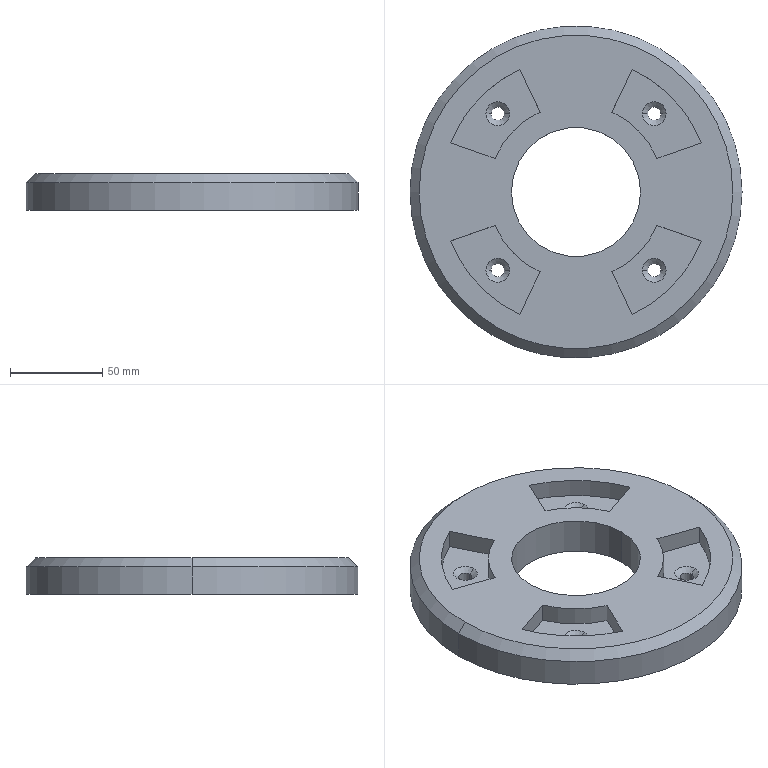Part | SolidWorks | features MirrorPattern 2, Chamfer 1, Extrusion 1, HoleWzd 1, ICE 1 | 1 solid | 44 faces | box 180 x 180 x 20 mm | volume 376159 mm3 | cylinder 20 | plane 14 | cone 10 | commonest cylinder face diameters 7.142 x8 95 x4 146.043 x4 70 x2 180 x2
STEP:
#1=CARTESIAN_POINT('',(38.855,-42.426,7.594));
#2=VERTEX_POINT('',#1);
#3=CARTESIAN_POINT('',(45.998,-42.426,7.594));
#4=VERTEX_POINT('',#3);
#5=CARTESIAN_POINT('',(42.426,-42.426,7.594));
#6=DIRECTION('',(0.,0.,1.));
#7=DIRECTION('',(1.,0.,0.));
#8=AXIS2_PLACEMENT_3D('',#5,#6,#7);
#9=CIRCLE('',#8,3.571);
#10=EDGE_CURVE('',#2,#4,#9,.T.);
#11=ORIENTED_EDGE('',*,*,#10,.F.);
#12=CARTESIAN_POINT('',(35.988,-42.426,10.));
#13=VERTEX_POINT('',#12);
#14=CARTESIAN_POINT('',(35.988,-42.426,10.));
#15=DIRECTION('',(-0.766,0.,0.6428));
#16=VECTOR('',#15,1000.);
#17=LINE('',#14,#16);
#18=EDGE_CURVE('',#2,#13,#17,.T.);
#19=ORIENTED_EDGE('',*,*,#18,.T.);
#20=CARTESIAN_POINT('',(48.865,-42.426,10.));
#21=VERTEX_POINT('',#20);
#22=CARTESIAN_POINT('',(42.426,-42.426,10.));
#23=DIRECTION('',(0.,0.,1.));
#24=DIRECTION('',(1.,0.,0.));
#25=AXIS2_PLACEMENT_3D('',#22,#23,#24);
#26=CIRCLE('',#25,6.439);
#27=EDGE_CURVE('',#13,#21,#26,.T.);
#28=ORIENTED_EDGE('',*,*,#27,.T.);
#29=CARTESIAN_POINT('',(48.865,-42.426,10.));
#30=DIRECTION('',(0.766,0.,0.6428));
#31=VECTOR('',#30,1000.);
#32=LINE('',#29,#31);
#33=EDGE_CURVE('',#4,#21,#32,.T.);
#34=ORIENTED_EDGE('',*,*,#33,.F.);
#35=EDGE_LOOP('',(#11,#19,#28,#34));
#36=FACE_OUTER_BOUND('',#35,.T.);
#37=CARTESIAN_POINT('',(42.426,-42.426,10.));
#38=DIRECTION('',(0.,0.,1.));
#39=DIRECTION('',(1.,0.,0.));
#40=AXIS2_PLACEMENT_3D('',#37,#38,#39);
#41=CONICAL_SURFACE('',#40,6.439,0.8727);
#42=ADVANCED_FACE('',(#36),#41,.F.);
#43=CARTESIAN_POINT('',(38.855,-42.426,0.));
#44=VERTEX_POINT('',#43);
#45=CARTESIAN_POINT('',(45.998,-42.426,0.));
#46=VERTEX_POINT('',#45);
#47=CARTESIAN_POINT('',(42.426,-42.426,0.));
#48=DIRECTION('',(0.,0.,1.));
#49=DIRECTION('',(1.,0.,0.));
#50=AXIS2_PLACEMENT_3D('',#47,#48,#49);
#51=CIRCLE('',#50,3.571);
#52=EDGE_CURVE('',#44,#46,#51,.T.);
#53=ORIENTED_EDGE('',*,*,#52,.F.);
#54=CARTESIAN_POINT('',(38.855,-42.426,10.));
#55=DIRECTION('',(0.,0.,1.));
#56=VECTOR('',#55,1000.);
#57=LINE('',#54,#56);
#58=EDGE_CURVE('',#44,#2,#57,.T.);
#59=ORIENTED_EDGE('',*,*,#58,.T.);
#60=ORIENTED_EDGE('',*,*,#10,.T.);
#61=CARTESIAN_POINT('',(45.998,-42.426,10.));
#62=DIRECTION('',(0.,0.,1.));
#63=VECTOR('',#62,1000.);
#64=LINE('',#61,#63);
#65=EDGE_CURVE('',#46,#4,#64,.T.);
#66=ORIENTED_EDGE('',*,*,#65,.F.);
#67=EDGE_LOOP('',(#53,#59,#60,#66));
#68=FACE_OUTER_BOUND('',#67,.T.);
#69=CARTESIAN_POINT('',(42.426,-42.426,10.));
#70=DIRECTION('',(0.,0.,1.));
#71=DIRECTION('',(1.,0.,0.));
#72=AXIS2_PLACEMENT_3D('',#69,#70,#71);
#73=CYLINDRICAL_SURFACE('',#72,3.571);
#74=ADVANCED_FACE('',(#68),#73,.F.);
#75=CARTESIAN_POINT('',(-45.998,-42.426,7.594));
#76=VERTEX_POINT('',#75);
#77=CARTESIAN_POINT('',(-38.855,-42.426,7.594));
#78=VERTEX_POINT('',#77);
#79=CARTESIAN_POINT('',(-42.426,-42.426,7.594));
#80=DIRECTION('',(0.,0.,1.));
#81=DIRECTION('',(1.,0.,0.));
#82=AXIS2_PLACEMENT_3D('',#79,#80,#81);
#83=CIRCLE('',#82,3.571);
#84=EDGE_CURVE('',#76,#78,#83,.T.);
#85=ORIENTED_EDGE('',*,*,#84,.F.);
#86=CARTESIAN_POINT('',(-48.865,-42.426,10.));
#87=VERTEX_POINT('',#86);
#88=CARTESIAN_POINT('',(-48.865,-42.426,10.));
#89=DIRECTION('',(-0.766,0.,0.6428));
#90=VECTOR('',#89,1000.);
#91=LINE('',#88,#90);
#92=EDGE_CURVE('',#76,#87,#91,.T.);
#93=ORIENTED_EDGE('',*,*,#92,.T.);
#94=CARTESIAN_POINT('',(-35.988,-42.426,10.));
#95=VERTEX_POINT('',#94);
#96=CARTESIAN_POINT('',(-42.426,-42.426,10.));
#97=DIRECTION('',(0.,0.,1.));
#98=DIRECTION('',(1.,0.,0.));
#99=AXIS2_PLACEMENT_3D('',#96,#97,#98);
#100=CIRCLE('',#99,6.439);
#101=EDGE_CURVE('',#87,#95,#100,.T.);
#102=ORIENTED_EDGE('',*,*,#101,.T.);
#103=CARTESIAN_POINT('',(-35.988,-42.426,10.));
#104=DIRECTION('',(0.766,0.,0.6428));
#105=VECTOR('',#104,1000.);
#106=LINE('',#103,#105);
#107=EDGE_CURVE('',#78,#95,#106,.T.);
#108=ORIENTED_EDGE('',*,*,#107,.F.);
#109=EDGE_LOOP('',(#85,#93,#102,#108));
#110=FACE_OUTER_BOUND('',#109,.T.);
#111=CARTESIAN_POINT('',(-42.426,-42.426,10.));
#112=DIRECTION('',(0.,0.,1.));
#113=DIRECTION('',(1.,0.,0.));
#114=AXIS2_PLACEMENT_3D('',#111,#112,#113);
#115=CONICAL_SURFACE('',#114,6.439,0.8727);
#116=ADVANCED_FACE('',(#110),#115,.F.);
#117=CARTESIAN_POINT('',(-45.998,-42.426,0.));
#118=VERTEX_POINT('',#117);
#119=CARTESIAN_POINT('',(-38.855,-42.426,0.));
#120=VERTEX_POINT('',#119);
#121=CARTESIAN_POINT('',(-42.426,-42.426,0.));
#122=DIRECTION('',(0.,0.,1.));
#123=DIRECTION('',(1.,0.,0.));
#124=AXIS2_PLACEMENT_3D('',#121,#122,#123);
#125=CIRCLE('',#124,3.571);
#126=EDGE_CURVE('',#118,#120,#125,.T.);
#127=ORIENTED_EDGE('',*,*,#126,.F.);
#128=CARTESIAN_POINT('',(-45.998,-42.426,10.));
#129=DIRECTION('',(0.,0.,1.));
#130=VECTOR('',#129,1000.);
#131=LINE('',#128,#130);
#132=EDGE_CURVE('',#118,#76,#131,.T.);
#133=ORIENTED_EDGE('',*,*,#132,.T.);
#134=ORIENTED_EDGE('',*,*,#84,.T.);
#135=CARTESIAN_POINT('',(-38.855,-42.426,10.));
#136=DIRECTION('',(0.,0.,1.));
#137=VECTOR('',#136,1000.);
#138=LINE('',#135,#137);
#139=EDGE_CURVE('',#120,#78,#138,.T.);
#140=ORIENTED_EDGE('',*,*,#139,.F.);
#141=EDGE_LOOP('',(#127,#133,#134,#140));
#142=FACE_OUTER_BOUND('',#141,.T.);
#143=CARTESIAN_POINT('',(-42.426,-42.426,10.));
#144=DIRECTION('',(0.,0.,1.));
#145=DIRECTION('',(1.,0.,0.));
#146=AXIS2_PLACEMENT_3D('',#143,#144,#145);
#147=CYLINDRICAL_SURFACE('',#146,3.571);
#148=ADVANCED_FACE('',(#142),#147,.F.);
#149=CARTESIAN_POINT('',(38.855,42.426,7.594));
#150=VERTEX_POINT('',#149);
#151=CARTESIAN_POINT('',(45.998,42.426,7.594));
#152=VERTEX_POINT('',#151);
#153=CARTESIAN_POINT('',(42.426,42.426,7.594));
#154=DIRECTION('',(0.,0.,1.));
#155=DIRECTION('',(1.,0.,0.));
#156=AXIS2_PLACEMENT_3D('',#153,#154,#155);
#157=CIRCLE('',#156,3.571);
#158=EDGE_CURVE('',#150,#152,#157,.T.);
#159=ORIENTED_EDGE('',*,*,#158,.F.);
#160=CARTESIAN_POINT('',(35.988,42.426,10.));
#161=VERTEX_POINT('',#160);
#162=CARTESIAN_POINT('',(35.988,42.426,10.));
#163=DIRECTION('',(-0.766,0.,0.6428));
#164=VECTOR('',#163,1000.);
#165=LINE('',#162,#164);
#166=EDGE_CURVE('',#150,#161,#165,.T.);
#167=ORIENTED_EDGE('',*,*,#166,.T.);
#168=CARTESIAN_POINT('',(48.865,42.426,10.));
#169=VERTEX_POINT('',#168);
#170=CARTESIAN_POINT('',(42.426,42.426,10.));
#171=DIRECTION('',(0.,0.,1.));
#172=DIRECTION('',(1.,0.,0.));
#173=AXIS2_PLACEMENT_3D('',#170,#171,#172);
#174=CIRCLE('',#173,6.439);
#175=EDGE_CURVE('',#161,#169,#174,.T.);
#176=ORIENTED_EDGE('',*,*,#175,.T.);
#177=CARTESIAN_POINT('',(48.865,42.426,10.));
#178=DIRECTION('',(0.766,0.,0.6428));
#179=VECTOR('',#178,1000.);
#180=LINE('',#177,#179);
#181=EDGE_CURVE('',#152,#169,#180,.T.);
#182=ORIENTED_EDGE('',*,*,#181,.F.);
#183=EDGE_LOOP('',(#159,#167,#176,#182));
#184=FACE_OUTER_BOUND('',#183,.T.);
#185=CARTESIAN_POINT('',(42.426,42.426,10.));
#186=DIRECTION('',(0.,0.,1.));
#187=DIRECTION('',(1.,0.,0.));
#188=AXIS2_PLACEMENT_3D('',#185,#186,#187);
#189=CONICAL_SURFACE('',#188,6.439,0.8727);
#190=ADVANCED_FACE('',(#184),#189,.F.);
#191=CARTESIAN_POINT('',(38.855,42.426,0.));
#192=VERTEX_POINT('',#191);
#193=CARTESIAN_POINT('',(45.998,42.426,0.));
#194=VERTEX_POINT('',#193);
#195=CARTESIAN_POINT('',(42.426,42.426,0.));
#196=DIRECTION('',(0.,0.,1.));
#197=DIRECTION('',(1.,0.,0.));
#198=AXIS2_PLACEMENT_3D('',#195,#196,#197);
#199=CIRCLE('',#198,3.571);
#200=EDGE_CURVE('',#192,#194,#199,.T.);
#201=ORIENTED_EDGE('',*,*,#200,.F.);
#202=CARTESIAN_POINT('',(38.855,42.426,10.));
#203=DIRECTION('',(0.,0.,1.));
#204=VECTOR('',#203,1000.);
#205=LINE('',#202,#204);
#206=EDGE_CURVE('',#192,#150,#205,.T.);
#207=ORIENTED_EDGE('',*,*,#206,.T.);
#208=ORIENTED_EDGE('',*,*,#158,.T.);
#209=CARTESIAN_POINT('',(45.998,42.426,10.));
#210=DIRECTION('',(0.,0.,1.));
#211=VECTOR('',#210,1000.);
#212=LINE('',#209,#211);
#213=EDGE_CURVE('',#194,#152,#212,.T.);
#214=ORIENTED_EDGE('',*,*,#213,.F.);
#215=EDGE_LOOP('',(#201,#207,#208,#214));
#216=FACE_OUTER_BOUND('',#215,.T.);
#217=CARTESIAN_POINT('',(42.426,42.426,10.));
#218=DIRECTION('',(0.,0.,1.));
#219=DIRECTION('',(1.,0.,0.));
#220=AXIS2_PLACEMENT_3D('',#217,#218,#219);
#221=CYLINDRICAL_SURFACE('',#220,3.571);
#222=ADVANCED_FACE('',(#216),#221,.F.);
#223=CARTESIAN_POINT('',(-45.998,42.426,7.594));
#224=VERTEX_POINT('',#223);
#225=CARTESIAN_POINT('',(-38.855,42.426,7.594));
#226=VERTEX_POINT('',#225);
#227=CARTESIAN_POINT('',(-42.426,42.426,7.594));
#228=DIRECTION('',(0.,0.,1.));
#229=DIRECTION('',(1.,0.,0.));
#230=AXIS2_PLACEMENT_3D('',#227,#228,#229);
#231=CIRCLE('',#230,3.571);
#232=EDGE_CURVE('',#224,#226,#231,.T.);
#233=ORIENTED_EDGE('',*,*,#232,.F.);
#234=CARTESIAN_POINT('',(-48.865,42.426,10.));
#235=VERTEX_POINT('',#234);
#236=CARTESIAN_POINT('',(-48.865,42.426,10.));
#237=DIRECTION('',(-0.766,0.,0.6428));
#238=VECTOR('',#237,1000.);
#239=LINE('',#236,#238);
#240=EDGE_CURVE('',#224,#235,#239,.T.);
#241=ORIENTED_EDGE('',*,*,#240,.T.);
#242=CARTESIAN_POINT('',(-35.988,42.426,10.));
#243=VERTEX_POINT('',#242);
#244=CARTESIAN_POINT('',(-42.426,42.426,10.));
#245=DIRECTION('',(0.,0.,1.));
#246=DIRECTION('',(1.,0.,0.));
#247=AXIS2_PLACEMENT_3D('',#244,#245,#246);
#248=CIRCLE('',#247,6.439);
#249=EDGE_CURVE('',#235,#243,#248,.T.);
#250=ORIENTED_EDGE('',*,*,#249,.T.);
#251=CARTESIAN_POINT('',(-35.988,42.426,10.));
#252=DIRECTION('',(0.766,0.,0.6428));
#253=VECTOR('',#252,1000.);
#254=LINE('',#251,#253);
#255=EDGE_CURVE('',#226,#243,#254,.T.);
#256=ORIENTED_EDGE('',*,*,#255,.F.);
#257=EDGE_LOOP('',(#233,#241,#250,#256));
#258=FACE_OUTER_BOUND('',#257,.T.);
#259=CARTESIAN_POINT('',(-42.426,42.426,10.));
#260=DIRECTION('',(0.,0.,1.));
#261=DIRECTION('',(1.,0.,0.));
#262=AXIS2_PLACEMENT_3D('',#259,#260,#261);
#263=CONICAL_SURFACE('',#262,6.439,0.8727);
#264=ADVANCED_FACE('',(#258),#263,.F.);
#265=CARTESIAN_POINT('',(-45.998,42.426,0.));
#266=VERTEX_POINT('',#265);
#267=CARTESIAN_POINT('',(-38.855,42.426,0.));
#268=VERTEX_POINT('',#267);
#269=CARTESIAN_POINT('',(-42.426,42.426,0.));
#270=DIRECTION('',(0.,0.,1.));
#271=DIRECTION('',(1.,0.,0.));
#272=AXIS2_PLACEMENT_3D('',#269,#270,#271);
#273=CIRCLE('',#272,3.571);
#274=EDGE_CURVE('',#266,#268,#273,.T.);
#275=ORIENTED_EDGE('',*,*,#274,.F.);
#276=CARTESIAN_POINT('',(-45.998,42.426,10.));
#277=DIRECTION('',(0.,0.,1.));
#278=VECTOR('',#277,1000.);
#279=LINE('',#276,#278);
#280=EDGE_CURVE('',#266,#224,#279,.T.);
#281=ORIENTED_EDGE('',*,*,#280,.T.);
#282=ORIENTED_EDGE('',*,*,#232,.T.);
#283=CARTESIAN_POINT('',(-38.855,42.426,10.));
#284=DIRECTION('',(0.,0.,1.));
#285=VECTOR('',#284,1000.);
#286=LINE('',#283,#285);
#287=EDGE_CURVE('',#268,#226,#286,.T.);
#288=ORIENTED_EDGE('',*,*,#287,.F.);
#289=EDGE_LOOP('',(#275,#281,#282,#288));
#290=FACE_OUTER_BOUND('',#289,.T.);
#291=CARTESIAN_POINT('',(-42.426,42.426,10.));
#292=DIRECTION('',(0.,0.,1.));
#293=DIRECTION('',(1.,0.,0.));
#294=AXIS2_PLACEMENT_3D('',#291,#292,#293);
#295=CYLINDRICAL_SURFACE('',#294,3.571);
#296=ADVANCED_FACE('',(#290),#295,.F.);
#297=CARTESIAN_POINT('',(85.,0.,20.));
#298=VERTEX_POINT('',#297);
#299=CARTESIAN_POINT('',(-85.,0.,20.));
#300=VERTEX_POINT('',#299);
#301=CARTESIAN_POINT('',(0.,0.,20.));
#302=DIRECTION('',(0.,0.,1.));
#303=DIRECTION('',(1.,0.,0.));
#304=AXIS2_PLACEMENT_3D('',#301,#302,#303);
#305=CIRCLE('',#304,85.);
#306=EDGE_CURVE('',#298,#300,#305,.T.);
#307=ORIENTED_EDGE('',*,*,#306,.F.);
#308=CARTESIAN_POINT('',(90.,0.,15.));
#309=VERTEX_POINT('',#308);
#310=CARTESIAN_POINT('',(85.,0.,20.));
#311=DIRECTION('',(0.7071,0.,-0.7071));
#312=VECTOR('',#311,1000.);
#313=LINE('',#310,#312);
#314=EDGE_CURVE('',#298,#309,#313,.T.);
#315=ORIENTED_EDGE('',*,*,#314,.T.);
#316=CARTESIAN_POINT('',(-90.,0.,15.));
#317=VERTEX_POINT('',#316);
#318=CARTESIAN_POINT('',(0.,0.,15.));
#319=DIRECTION('',(0.,0.,-1.));
#320=DIRECTION('',(1.,0.,0.));
#321=AXIS2_PLACEMENT_3D('',#318,#319,#320);
#322=CIRCLE('',#321,90.);
#323=EDGE_CURVE('',#317,#309,#322,.T.);
#324=ORIENTED_EDGE('',*,*,#323,.F.);
#325=CARTESIAN_POINT('',(-85.,0.,20.));
#326=DIRECTION('',(-0.7071,0.,-0.7071));
#327=VECTOR('',#326,1000.);
#328=LINE('',#325,#327);
#329=EDGE_CURVE('',#300,#317,#328,.T.);
#330=ORIENTED_EDGE('',*,*,#329,.F.);
#331=EDGE_LOOP('',(#307,#315,#324,#330));
#332=FACE_OUTER_BOUND('',#331,.T.);
#333=CARTESIAN_POINT('',(0.,0.,20.));
#334=DIRECTION('',(0.,0.,-1.));
#335=DIRECTION('',(-1.,0.,0.));
#336=AXIS2_PLACEMENT_3D('',#333,#334,#335);
#337=CONICAL_SURFACE('',#336,85.,0.7854);
#338=ADVANCED_FACE('',(#332),#337,.T.);
#339=CARTESIAN_POINT('',(-35.,0.,20.));
#340=VERTEX_POINT('',#339);
#341=CARTESIAN_POINT('',(35.,0.,20.));
#342=VERTEX_POINT('',#341);
#343=CARTESIAN_POINT('',(0.,0.,20.));
#344=DIRECTION('',(0.,0.,1.));
#345=DIRECTION('',(1.,0.,0.));
#346=AXIS2_PLACEMENT_3D('',#343,#344,#345);
#347=CIRCLE('',#346,35.);
#348=EDGE_CURVE('',#340,#342,#347,.T.);
#349=ORIENTED_EDGE('',*,*,#348,.T.);
#350=CARTESIAN_POINT('',(35.,0.,0.));
#351=VERTEX_POINT('',#350);
#352=CARTESIAN_POINT('',(35.,0.,20.));
#353=DIRECTION('',(0.,0.,-1.));
#354=VECTOR('',#353,1000.);
#355=LINE('',#352,#354);
#356=EDGE_CURVE('',#342,#351,#355,.T.);
#357=ORIENTED_EDGE('',*,*,#356,.T.);
#358=CARTESIAN_POINT('',(-35.,0.,0.));
#359=VERTEX_POINT('',#358);
#360=CARTESIAN_POINT('',(0.,0.,0.));
#361=DIRECTION('',(0.,0.,1.));
#362=DIRECTION('',(1.,0.,0.));
#363=AXIS2_PLACEMENT_3D('',#360,#361,#362);
#364=CIRCLE('',#363,35.);
#365=EDGE_CURVE('',#359,#351,#364,.T.);
#366=ORIENTED_EDGE('',*,*,#365,.F.);
#367=CARTESIAN_POINT('',(-35.,0.,20.));
#368=DIRECTION('',(0.,0.,-1.));
#369=VECTOR('',#368,1000.);
#370=LINE('',#367,#369);
#371=EDGE_CURVE('',#340,#359,#370,.T.);
#372=ORIENTED_EDGE('',*,*,#371,.F.);
#373=EDGE_LOOP('',(#349,#357,#366,#372));
#374=FACE_OUTER_BOUND('',#373,.T.);
#375=CARTESIAN_POINT('',(0.,0.,20.));
#376=DIRECTION('',(0.,0.,-1.));
#377=DIRECTION('',(-1.,0.,0.));
#378=AXIS2_PLACEMENT_3D('',#375,#376,#377);
#379=CYLINDRICAL_SURFACE('',#378,35.);
#380=ADVANCED_FACE('',(#374),#379,.F.);
#381=ORIENTED_EDGE('',*,*,#323,.T.);
#382=CARTESIAN_POINT('',(90.,0.,0.));
#383=VERTEX_POINT('',#382);
#384=CARTESIAN_POINT('',(90.,0.,20.));
#385=DIRECTION('',(0.,0.,-1.));
#386=VECTOR('',#385,1000.);
#387=LINE('',#384,#386);
#388=EDGE_CURVE('',#309,#383,#387,.T.);
#389=ORIENTED_EDGE('',*,*,#388,.T.);
#390=CARTESIAN_POINT('',(-90.,0.,0.));
#391=VERTEX_POINT('',#390);
#392=CARTESIAN_POINT('',(0.,0.,0.));
#393=DIRECTION('',(0.,0.,1.));
#394=DIRECTION('',(1.,0.,0.));
#395=AXIS2_PLACEMENT_3D('',#392,#393,#394);
#396=CIRCLE('',#395,90.);
#397=EDGE_CURVE('',#383,#391,#396,.T.);
#398=ORIENTED_EDGE('',*,*,#397,.T.);
#399=CARTESIAN_POINT('',(-90.,0.,20.));
#400=DIRECTION('',(0.,0.,-1.));
#401=VECTOR('',#400,1000.);
#402=LINE('',#399,#401);
#403=EDGE_CURVE('',#317,#391,#402,.T.);
#404=ORIENTED_EDGE('',*,*,#403,.F.);
#405=EDGE_LOOP('',(#381,#389,#398,#404));
#406=FACE_OUTER_BOUND('',#405,.T.);
#407=CARTESIAN_POINT('',(0.,0.,20.));
#408=DIRECTION('',(0.,0.,-1.));
#409=DIRECTION('',(-1.,0.,0.));
#410=AXIS2_PLACEMENT_3D('',#407,#408,#409);
#411=CYLINDRICAL_SURFACE('',#410,90.);
#412=ADVANCED_FACE('',(#406),#411,.T.);
#413=CARTESIAN_POINT('',(0.,0.,20.));
#414=DIRECTION('',(0.,0.,1.));
#415=DIRECTION('',(1.,0.,0.));
#416=AXIS2_PLACEMENT_3D('',#413,#414,#415);
#417=CIRCLE('',#416,85.);
#418=EDGE_CURVE('',#300,#298,#417,.T.);
#419=ORIENTED_EDGE('',*,*,#418,.T.);
#420=ORIENTED_EDGE('',*,*,#306,.T.);
#421=EDGE_LOOP('',(#419,#420));
#422=FACE_OUTER_BOUND('',#421,.T.);
#423=CARTESIAN_POINT('',(-19.468,-43.327,20.));
#424=VERTEX_POINT('',#423);
#425=CARTESIAN_POINT('',(-43.883,-18.181,20.));
#426=VERTEX_POINT('',#425);
#427=CARTESIAN_POINT('',(0.,0.,20.));
#428=DIRECTION('',(0.,0.,-1.));
#429=DIRECTION('',(1.,0.,0.));
#430=AXIS2_PLACEMENT_3D('',#427,#428,#429);
#431=CIRCLE('',#430,47.5);
#432=EDGE_CURVE('',#424,#426,#431,.T.);
#433=ORIENTED_EDGE('',*,*,#432,.F.);
#434=CARTESIAN_POINT('',(-30.542,-66.327,20.));
#435=VERTEX_POINT('',#434);
#436=CARTESIAN_POINT('',(-19.468,-43.327,20.));
#437=DIRECTION('',(0.4338,0.901,0.));
#438=VECTOR('',#437,1000.);
#439=LINE('',#436,#438);
#440=EDGE_CURVE('',#435,#424,#439,.T.);
#441=ORIENTED_EDGE('',*,*,#440,.F.);
#442=CARTESIAN_POINT('',(-67.996,-26.621,20.));
#443=VERTEX_POINT('',#442);
#444=CARTESIAN_POINT('',(0.,0.,20.));
#445=DIRECTION('',(0.,0.,1.));
#446=DIRECTION('',(-1.,0.,0.));
#447=AXIS2_PLACEMENT_3D('',#444,#445,#446);
#448=CIRCLE('',#447,73.022);
#449=EDGE_CURVE('',#443,#435,#448,.T.);
#450=ORIENTED_EDGE('',*,*,#449,.F.);
#451=CARTESIAN_POINT('',(-43.883,-18.181,20.));
#452=DIRECTION('',(-0.9439,-0.3304,0.));
#453=VECTOR('',#452,1000.);
#454=LINE('',#451,#453);
#455=EDGE_CURVE('',#426,#443,#454,.T.);
#456=ORIENTED_EDGE('',*,*,#455,.F.);
#457=EDGE_LOOP('',(#433,#441,#450,#456));
#458=FACE_BOUND('',#457,.T.);
#459=CARTESIAN_POINT('',(43.883,-18.181,20.));
#460=VERTEX_POINT('',#459);
#461=CARTESIAN_POINT('',(19.468,-43.327,20.));
#462=VERTEX_POINT('',#461);
#463=CARTESIAN_POINT('',(0.,0.,20.));
#464=DIRECTION('',(0.,0.,-1.));
#465=DIRECTION('',(1.,0.,0.));
#466=AXIS2_PLACEMENT_3D('',#463,#464,#465);
#467=CIRCLE('',#466,47.5);
#468=EDGE_CURVE('',#460,#462,#467,.T.);
#469=ORIENTED_EDGE('',*,*,#468,.F.);
#470=CARTESIAN_POINT('',(67.996,-26.621,20.));
#471=VERTEX_POINT('',#470);
#472=CARTESIAN_POINT('',(43.883,-18.181,20.));
#473=DIRECTION('',(-0.9439,0.3304,0.));
#474=VECTOR('',#473,1000.);
#475=LINE('',#472,#474);
#476=EDGE_CURVE('',#471,#460,#475,.T.);
#477=ORIENTED_EDGE('',*,*,#476,.F.);
#478=CARTESIAN_POINT('',(30.542,-66.327,20.));
#479=VERTEX_POINT('',#478);
#480=CARTESIAN_POINT('',(0.,0.,20.));
#481=DIRECTION('',(0.,0.,1.));
#482=DIRECTION('',(1.,0.,0.));
#483=AXIS2_PLACEMENT_3D('',#480,#481,#482);
#484=CIRCLE('',#483,73.022);
#485=EDGE_CURVE('',#479,#471,#484,.T.);
#486=ORIENTED_EDGE('',*,*,#485,.F.);
#487=CARTESIAN_POINT('',(19.468,-43.327,20.));
#488=DIRECTION('',(0.4338,-0.901,0.));
#489=VECTOR('',#488,1000.);
#490=LINE('',#487,#489);
#491=EDGE_CURVE('',#462,#479,#490,.T.);
#492=ORIENTED_EDGE('',*,*,#491,.F.);
#493=EDGE_LOOP('',(#469,#477,#486,#492));
#494=FACE_BOUND('',#493,.T.);
#495=CARTESIAN_POINT('',(-43.883,18.181,20.));
#496=VERTEX_POINT('',#495);
#497=CARTESIAN_POINT('',(-19.468,43.327,20.));
#498=VERTEX_POINT('',#497);
#499=CARTESIAN_POINT('',(0.,0.,20.));
#500=DIRECTION('',(0.,0.,-1.));
#501=DIRECTION('',(1.,0.,0.));
#502=AXIS2_PLACEMENT_3D('',#499,#500,#501);
#503=CIRCLE('',#502,47.5);
#504=EDGE_CURVE('',#496,#498,#503,.T.);
#505=ORIENTED_EDGE('',*,*,#504,.F.);
#506=CARTESIAN_POINT('',(-67.996,26.621,20.));
#507=VERTEX_POINT('',#506);
#508=CARTESIAN_POINT('',(-43.883,18.181,20.));
#509=DIRECTION('',(0.9439,-0.3304,0.));
#510=VECTOR('',#509,1000.);
#511=LINE('',#508,#510);
#512=EDGE_CURVE('',#507,#496,#511,.T.);
#513=ORIENTED_EDGE('',*,*,#512,.F.);
#514=CARTESIAN_POINT('',(-30.542,66.327,20.));
#515=VERTEX_POINT('',#514);
#516=CARTESIAN_POINT('',(0.,0.,20.));
#517=DIRECTION('',(0.,0.,1.));
#518=DIRECTION('',(1.,0.,0.));
#519=AXIS2_PLACEMENT_3D('',#516,#517,#518);
#520=CIRCLE('',#519,73.022);
#521=EDGE_CURVE('',#515,#507,#520,.T.);
#522=ORIENTED_EDGE('',*,*,#521,.F.);
#523=CARTESIAN_POINT('',(-19.468,43.327,20.));
#524=DIRECTION('',(-0.4338,0.901,0.));
#525=VECTOR('',#524,1000.);
#526=LINE('',#523,#525);
#527=EDGE_CURVE('',#498,#515,#526,.T.);
#528=ORIENTED_EDGE('',*,*,#527,.F.);
#529=EDGE_LOOP('',(#505,#513,#522,#528));
#530=FACE_BOUND('',#529,.T.);
#531=CARTESIAN_POINT('',(19.468,43.327,20.));
#532=VERTEX_POINT('',#531);
#533=CARTESIAN_POINT('',(43.883,18.181,20.));
#534=VERTEX_POINT('',#533);
#535=CARTESIAN_POINT('',(0.,0.,20.));
#536=DIRECTION('',(0.,0.,-1.));
#537=DIRECTION('',(1.,0.,0.));
#538=AXIS2_PLACEMENT_3D('',#535,#536,#537);
#539=CIRCLE('',#538,47.5);
#540=EDGE_CURVE('',#532,#534,#539,.T.);
#541=ORIENTED_EDGE('',*,*,#540,.F.);
#542=CARTESIAN_POINT('',(30.542,66.327,20.));
#543=VERTEX_POINT('',#542);
#544=CARTESIAN_POINT('',(19.468,43.327,20.));
#545=DIRECTION('',(-0.4338,-0.901,0.));
#546=VECTOR('',#545,1000.);
#547=LINE('',#544,#546);
#548=EDGE_CURVE('',#543,#532,#547,.T.);
#549=ORIENTED_EDGE('',*,*,#548,.F.);
#550=CARTESIAN_POINT('',(67.996,26.621,20.));
#551=VERTEX_POINT('',#550);
#552=CARTESIAN_POINT('',(0.,0.,20.));
#553=DIRECTION('',(0.,0.,1.));
#554=DIRECTION('',(-1.,0.,0.));
#555=AXIS2_PLACEMENT_3D('',#552,#553,#554);
#556=CIRCLE('',#555,73.022);
#557=EDGE_CURVE('',#551,#543,#556,.T.);
#558=ORIENTED_EDGE('',*,*,#557,.F.);
#559=CARTESIAN_POINT('',(43.883,18.181,20.));
#560=DIRECTION('',(0.9439,0.3304,0.));
#561=VECTOR('',#560,1000.);
#562=LINE('',#559,#561);
#563=EDGE_CURVE('',#534,#551,#562,.T.);
#564=ORIENTED_EDGE('',*,*,#563,.F.);
#565=EDGE_LOOP('',(#541,#549,#558,#564));
#566=FACE_BOUND('',#565,.T.);
#567=ORIENTED_EDGE('',*,*,#348,.F.);
#568=CARTESIAN_POINT('',(0.,0.,20.));
#569=DIRECTION('',(0.,0.,1.));
#570=DIRECTION('',(1.,0.,0.));
#571=AXIS2_PLACEMENT_3D('',#568,#569,#570);
#572=CIRCLE('',#571,35.);
#573=EDGE_CURVE('',#342,#340,#572,.T.);
#574=ORIENTED_EDGE('',*,*,#573,.F.);
#575=EDGE_LOOP('',(#567,#574));
#576=FACE_BOUND('',#575,.T.);
#577=CARTESIAN_POINT('',(0.,0.,20.));
#578=DIRECTION('',(0.,0.,1.));
#579=DIRECTION('',(1.,0.,0.));
#580=AXIS2_PLACEMENT_3D('',#577,#578,#579);
#581=PLANE('',#580);
#582=ADVANCED_FACE('',(#422,#458,#494,#530,#566,#576),#581,.T.);
#583=CARTESIAN_POINT('',(42.426,-42.426,0.));
#584=DIRECTION('',(0.,0.,1.));
#585=DIRECTION('',(1.,0.,0.));
#586=AXIS2_PLACEMENT_3D('',#583,#584,#585);
#587=CIRCLE('',#586,3.571);
#588=EDGE_CURVE('',#46,#44,#587,.T.);
#589=ORIENTED_EDGE('',*,*,#588,.T.);
#590=ORIENTED_EDGE('',*,*,#52,.T.);
#591=EDGE_LOOP('',(#589,#590));
#592=FACE_BOUND('',#591,.T.);
#593=CARTESIAN_POINT('',(-42.426,-42.426,0.));
#594=DIRECTION('',(0.,0.,1.));
#595=DIRECTION('',(1.,0.,0.));
#596=AXIS2_PLACEMENT_3D('',#593,#594,#595);
#597=CIRCLE('',#596,3.571);
#598=EDGE_CURVE('',#120,#118,#597,.T.);
#599=ORIENTED_EDGE('',*,*,#598,.T.);
#600=ORIENTED_EDGE('',*,*,#126,.T.);
#601=EDGE_LOOP('',(#599,#600));
#602=FACE_BOUND('',#601,.T.);
#603=CARTESIAN_POINT('',(42.426,42.426,0.));
#604=DIRECTION('',(0.,0.,1.));
#605=DIRECTION('',(1.,0.,0.));
#606=AXIS2_PLACEMENT_3D('',#603,#604,#605);
#607=CIRCLE('',#606,3.571);
#608=EDGE_CURVE('',#194,#192,#607,.T.);
#609=ORIENTED_EDGE('',*,*,#608,.T.);
#610=ORIENTED_EDGE('',*,*,#200,.T.);
#611=EDGE_LOOP('',(#609,#610));
#612=FACE_BOUND('',#611,.T.);
#613=CARTESIAN_POINT('',(-42.426,42.426,0.));
#614=DIRECTION('',(0.,0.,1.));
#615=DIRECTION('',(1.,0.,0.));
#616=AXIS2_PLACEMENT_3D('',#613,#614,#615);
#617=CIRCLE('',#616,3.571);
#618=EDGE_CURVE('',#268,#266,#617,.T.);
#619=ORIENTED_EDGE('',*,*,#618,.T.);
#620=ORIENTED_EDGE('',*,*,#274,.T.);
#621=EDGE_LOOP('',(#619,#620));
#622=FACE_BOUND('',#621,.T.);
#623=CARTESIAN_POINT('',(0.,0.,0.));
#624=DIRECTION('',(0.,0.,1.));
#625=DIRECTION('',(1.,0.,0.));
#626=AXIS2_PLACEMENT_3D('',#623,#624,#625);
#627=CIRCLE('',#626,90.);
#628=EDGE_CURVE('',#391,#383,#627,.T.);
#629=ORIENTED_EDGE('',*,*,#628,.F.);
#630=ORIENTED_EDGE('',*,*,#397,.F.);
#631=EDGE_LOOP('',(#629,#630));
#632=FACE_OUTER_BOUND('',#631,.T.);
#633=ORIENTED_EDGE('',*,*,#365,.T.);
#634=CARTESIAN_POINT('',(0.,0.,0.));
#635=DIRECTION('',(0.,0.,1.));
#636=DIRECTION('',(1.,0.,0.));
#637=AXIS2_PLACEMENT_3D('',#634,#635,#636);
#638=CIRCLE('',#637,35.);
#639=EDGE_CURVE('',#351,#359,#638,.T.);
#640=ORIENTED_EDGE('',*,*,#639,.T.);
#641=EDGE_LOOP('',(#633,#640));
#642=FACE_BOUND('',#641,.T.);
#643=CARTESIAN_POINT('',(0.,0.,0.));
#644=DIRECTION('',(0.,0.,1.));
#645=DIRECTION('',(1.,0.,0.));
#646=AXIS2_PLACEMENT_3D('',#643,#644,#645);
#647=PLANE('',#646);
#648=ADVANCED_FACE('',(#592,#602,#612,#622,#632,#642),#647,.F.);
#649=ORIENTED_EDGE('',*,*,#388,.F.);
#650=CARTESIAN_POINT('',(0.,0.,15.));
#651=DIRECTION('',(0.,0.,-1.));
#652=DIRECTION('',(1.,0.,0.));
#653=AXIS2_PLACEMENT_3D('',#650,#651,#652);
#654=CIRCLE('',#653,90.);
#655=EDGE_CURVE('',#309,#317,#654,.T.);
#656=ORIENTED_EDGE('',*,*,#655,.T.);
#657=ORIENTED_EDGE('',*,*,#403,.T.);
#658=ORIENTED_EDGE('',*,*,#628,.T.);
#659=EDGE_LOOP('',(#649,#656,#657,#658));
#660=FACE_OUTER_BOUND('',#659,.T.);
#661=CARTESIAN_POINT('',(0.,0.,20.));
#662=DIRECTION('',(0.,0.,-1.));
#663=DIRECTION('',(-1.,0.,0.));
#664=AXIS2_PLACEMENT_3D('',#661,#662,#663);
#665=CYLINDRICAL_SURFACE('',#664,90.);
#666=ADVANCED_FACE('',(#660),#665,.T.);
#667=ORIENTED_EDGE('',*,*,#356,.F.);
#668=ORIENTED_EDGE('',*,*,#573,.T.);
#669=ORIENTED_EDGE('',*,*,#371,.T.);
#670=ORIENTED_EDGE('',*,*,#639,.F.);
#671=EDGE_LOOP('',(#667,#668,#669,#670));
#672=FACE_OUTER_BOUND('',#671,.T.);
#673=CARTESIAN_POINT('',(0.,0.,20.));
#674=DIRECTION('',(0.,0.,-1.));
#675=DIRECTION('',(-1.,0.,0.));
#676=AXIS2_PLACEMENT_3D('',#673,#674,#675);
#677=CYLINDRICAL_SURFACE('',#676,35.);
#678=ADVANCED_FACE('',(#672),#677,.F.);
#679=ORIENTED_EDGE('',*,*,#540,.T.);
#680=CARTESIAN_POINT('',(43.883,18.181,10.));
#681=VERTEX_POINT('',#680);
#682=CARTESIAN_POINT('',(43.883,18.181,10.));
#683=DIRECTION('',(0.,0.,1.));
#684=VECTOR('',#683,1000.);
#685=LINE('',#682,#684);
#686=EDGE_CURVE('',#681,#534,#685,.T.);
#687=ORIENTED_EDGE('',*,*,#686,.F.);
#688=CARTESIAN_POINT('',(19.468,43.327,10.));
#689=VERTEX_POINT('',#688);
#690=CARTESIAN_POINT('',(0.,0.,10.));
#691=DIRECTION('',(0.,0.,-1.));
#692=DIRECTION('',(1.,0.,0.));
#693=AXIS2_PLACEMENT_3D('',#690,#691,#692);
#694=CIRCLE('',#693,47.5);
#695=EDGE_CURVE('',#689,#681,#694,.T.);
#696=ORIENTED_EDGE('',*,*,#695,.F.);
#697=CARTESIAN_POINT('',(19.468,43.327,10.));
#698=DIRECTION('',(0.,0.,1.));
#699=VECTOR('',#698,1000.);
#700=LINE('',#697,#699);
#701=EDGE_CURVE('',#689,#532,#700,.T.);
#702=ORIENTED_EDGE('',*,*,#701,.T.);
#703=EDGE_LOOP('',(#679,#687,#696,#702));
#704=FACE_OUTER_BOUND('',#703,.T.);
#705=CARTESIAN_POINT('',(0.,0.,10.));
#706=DIRECTION('',(0.,0.,1.));
#707=DIRECTION('',(1.,0.,0.));
#708=AXIS2_PLACEMENT_3D('',#705,#706,#707);
#709=CYLINDRICAL_SURFACE('',#708,47.5);
#710=ADVANCED_FACE('',(#704),#709,.T.);
#711=ORIENTED_EDGE('',*,*,#548,.T.);
#712=ORIENTED_EDGE('',*,*,#701,.F.);
#713=CARTESIAN_POINT('',(30.542,66.327,10.));
#714=VERTEX_POINT('',#713);
#715=CARTESIAN_POINT('',(19.468,43.327,10.));
#716=DIRECTION('',(-0.4338,-0.901,0.));
#717=VECTOR('',#716,1000.);
#718=LINE('',#715,#717);
#719=EDGE_CURVE('',#714,#689,#718,.T.);
#720=ORIENTED_EDGE('',*,*,#719,.F.);
#721=CARTESIAN_POINT('',(30.542,66.327,10.));
#722=DIRECTION('',(0.,0.,1.));
#723=VECTOR('',#722,1000.);
#724=LINE('',#721,#723);
#725=EDGE_CURVE('',#714,#543,#724,.T.);
#726=ORIENTED_EDGE('',*,*,#725,.T.);
#727=EDGE_LOOP('',(#711,#712,#720,#726));
#728=FACE_OUTER_BOUND('',#727,.T.);
#729=CARTESIAN_POINT('',(19.468,43.327,10.));
#730=DIRECTION('',(-0.901,0.4338,0.));
#731=DIRECTION('',(-0.4338,-0.901,0.));
#732=AXIS2_PLACEMENT_3D('',#729,#730,#731);
#733=PLANE('',#732);
#734=ADVANCED_FACE('',(#728),#733,.F.);
#735=ORIENTED_EDGE('',*,*,#557,.T.);
#736=ORIENTED_EDGE('',*,*,#725,.F.);
#737=CARTESIAN_POINT('',(67.996,26.621,10.));
#738=VERTEX_POINT('',#737);
#739=CARTESIAN_POINT('',(0.,0.,10.));
#740=DIRECTION('',(0.,0.,1.));
#741=DIRECTION('',(-1.,0.,0.));
#742=AXIS2_PLACEMENT_3D('',#739,#740,#741);
#743=CIRCLE('',#742,73.022);
#744=EDGE_CURVE('',#738,#714,#743,.T.);
#745=ORIENTED_EDGE('',*,*,#744,.F.);
#746=CARTESIAN_POINT('',(67.996,26.621,10.));
#747=DIRECTION('',(0.,0.,1.));
#748=VECTOR('',#747,1000.);
#749=LINE('',#746,#748);
#750=EDGE_CURVE('',#738,#551,#749,.T.);
#751=ORIENTED_EDGE('',*,*,#750,.T.);
#752=EDGE_LOOP('',(#735,#736,#745,#751));
#753=FACE_OUTER_BOUND('',#752,.T.);
#754=CARTESIAN_POINT('',(0.,0.,10.));
#755=DIRECTION('',(0.,0.,1.));
#756=DIRECTION('',(1.,0.,0.));
#757=AXIS2_PLACEMENT_3D('',#754,#755,#756);
#758=CYLINDRICAL_SURFACE('',#757,73.022);
#759=ADVANCED_FACE('',(#753),#758,.F.);
#760=ORIENTED_EDGE('',*,*,#563,.T.);
#761=ORIENTED_EDGE('',*,*,#750,.F.);
#762=CARTESIAN_POINT('',(43.883,18.181,10.));
#763=DIRECTION('',(0.9439,0.3304,0.));
#764=VECTOR('',#763,1000.);
#765=LINE('',#762,#764);
#766=EDGE_CURVE('',#681,#738,#765,.T.);
#767=ORIENTED_EDGE('',*,*,#766,.F.);
#768=ORIENTED_EDGE('',*,*,#686,.T.);
#769=EDGE_LOOP('',(#760,#761,#767,#768));
#770=FACE_OUTER_BOUND('',#769,.T.);
#771=CARTESIAN_POINT('',(43.883,18.181,10.));
#772=DIRECTION('',(0.3304,-0.9439,0.));
#773=DIRECTION('',(0.9439,0.3304,0.));
#774=AXIS2_PLACEMENT_3D('',#771,#772,#773);
#775=PLANE('',#774);
#776=ADVANCED_FACE('',(#770),#775,.F.);
#777=CARTESIAN_POINT('',(42.426,42.426,10.));
#778=DIRECTION('',(0.,0.,1.));
#779=DIRECTION('',(1.,0.,0.));
#780=AXIS2_PLACEMENT_3D('',#777,#778,#779);
#781=CIRCLE('',#780,6.439);
#782=EDGE_CURVE('',#169,#161,#781,.T.);
#783=ORIENTED_EDGE('',*,*,#782,.F.);
#784=ORIENTED_EDGE('',*,*,#175,.F.);
#785=EDGE_LOOP('',(#783,#784));
#786=FACE_BOUND('',#785,.T.);
#787=ORIENTED_EDGE('',*,*,#695,.T.);
#788=ORIENTED_EDGE('',*,*,#766,.T.);
#789=ORIENTED_EDGE('',*,*,#744,.T.);
#790=ORIENTED_EDGE('',*,*,#719,.T.);
#791=EDGE_LOOP('',(#787,#788,#789,#790));
#792=FACE_OUTER_BOUND('',#791,.T.);
#793=CARTESIAN_POINT('',(0.,0.,10.));
#794=DIRECTION('',(0.,0.,1.));
#795=DIRECTION('',(1.,0.,0.));
#796=AXIS2_PLACEMENT_3D('',#793,#794,#795);
#797=PLANE('',#796);
#798=ADVANCED_FACE('',(#786,#792),#797,.T.);
#799=ORIENTED_EDGE('',*,*,#504,.T.);
#800=CARTESIAN_POINT('',(-19.468,43.327,10.));
#801=VERTEX_POINT('',#800);
#802=CARTESIAN_POINT('',(-19.468,43.327,10.));
#803=DIRECTION('',(0.,0.,1.));
#804=VECTOR('',#803,1000.);
#805=LINE('',#802,#804);
#806=EDGE_CURVE('',#801,#498,#805,.T.);
#807=ORIENTED_EDGE('',*,*,#806,.F.);
#808=CARTESIAN_POINT('',(-43.883,18.181,10.));
#809=VERTEX_POINT('',#808);
#810=CARTESIAN_POINT('',(0.,0.,10.));
#811=DIRECTION('',(0.,0.,-1.));
#812=DIRECTION('',(1.,0.,0.));
#813=AXIS2_PLACEMENT_3D('',#810,#811,#812);
#814=CIRCLE('',#813,47.5);
#815=EDGE_CURVE('',#809,#801,#814,.T.);
#816=ORIENTED_EDGE('',*,*,#815,.F.);
#817=CARTESIAN_POINT('',(-43.883,18.181,10.));
#818=DIRECTION('',(0.,0.,1.));
#819=VECTOR('',#818,1000.);
#820=LINE('',#817,#819);
#821=EDGE_CURVE('',#809,#496,#820,.T.);
#822=ORIENTED_EDGE('',*,*,#821,.T.);
#823=EDGE_LOOP('',(#799,#807,#816,#822));
#824=FACE_OUTER_BOUND('',#823,.T.);
#825=CARTESIAN_POINT('',(0.,0.,10.));
#826=DIRECTION('',(0.,0.,1.));
#827=DIRECTION('',(1.,0.,0.));
#828=AXIS2_PLACEMENT_3D('',#825,#826,#827);
#829=CYLINDRICAL_SURFACE('',#828,47.5);
#830=ADVANCED_FACE('',(#824),#829,.T.);
#831=ORIENTED_EDGE('',*,*,#512,.T.);
#832=ORIENTED_EDGE('',*,*,#821,.F.);
#833=CARTESIAN_POINT('',(-67.996,26.621,10.));
#834=VERTEX_POINT('',#833);
#835=CARTESIAN_POINT('',(-43.883,18.181,10.));
#836=DIRECTION('',(0.9439,-0.3304,0.));
#837=VECTOR('',#836,1000.);
#838=LINE('',#835,#837);
#839=EDGE_CURVE('',#834,#809,#838,.T.);
#840=ORIENTED_EDGE('',*,*,#839,.F.);
#841=CARTESIAN_POINT('',(-67.996,26.621,10.));
#842=DIRECTION('',(0.,0.,1.));
#843=VECTOR('',#842,1000.);
#844=LINE('',#841,#843);
#845=EDGE_CURVE('',#834,#507,#844,.T.);
#846=ORIENTED_EDGE('',*,*,#845,.T.);
#847=EDGE_LOOP('',(#831,#832,#840,#846));
#848=FACE_OUTER_BOUND('',#847,.T.);
#849=CARTESIAN_POINT('',(-43.883,18.181,10.));
#850=DIRECTION('',(-0.3304,-0.9439,0.));
#851=DIRECTION('',(0.9439,-0.3304,0.));
#852=AXIS2_PLACEMENT_3D('',#849,#850,#851);
#853=PLANE('',#852);
#854=ADVANCED_FACE('',(#848),#853,.F.);
#855=ORIENTED_EDGE('',*,*,#521,.T.);
#856=ORIENTED_EDGE('',*,*,#845,.F.);
#857=CARTESIAN_POINT('',(-30.542,66.327,10.));
#858=VERTEX_POINT('',#857);
#859=CARTESIAN_POINT('',(0.,0.,10.));
#860=DIRECTION('',(0.,0.,1.));
#861=DIRECTION('',(1.,0.,0.));
#862=AXIS2_PLACEMENT_3D('',#859,#860,#861);
#863=CIRCLE('',#862,73.022);
#864=EDGE_CURVE('',#858,#834,#863,.T.);
#865=ORIENTED_EDGE('',*,*,#864,.F.);
#866=CARTESIAN_POINT('',(-30.542,66.327,10.));
#867=DIRECTION('',(0.,0.,1.));
#868=VECTOR('',#867,1000.);
#869=LINE('',#866,#868);
#870=EDGE_CURVE('',#858,#515,#869,.T.);
#871=ORIENTED_EDGE('',*,*,#870,.T.);
#872=EDGE_LOOP('',(#855,#856,#865,#871));
#873=FACE_OUTER_BOUND('',#872,.T.);
#874=CARTESIAN_POINT('',(0.,0.,10.));
#875=DIRECTION('',(0.,0.,1.));
#876=DIRECTION('',(1.,0.,0.));
#877=AXIS2_PLACEMENT_3D('',#874,#875,#876);
#878=CYLINDRICAL_SURFACE('',#877,73.022);
#879=ADVANCED_FACE('',(#873),#878,.F.);
#880=ORIENTED_EDGE('',*,*,#527,.T.);
#881=ORIENTED_EDGE('',*,*,#870,.F.);
#882=CARTESIAN_POINT('',(-19.468,43.327,10.));
#883=DIRECTION('',(-0.4338,0.901,0.));
#884=VECTOR('',#883,1000.);
#885=LINE('',#882,#884);
#886=EDGE_CURVE('',#801,#858,#885,.T.);
#887=ORIENTED_EDGE('',*,*,#886,.F.);
#888=ORIENTED_EDGE('',*,*,#806,.T.);
#889=EDGE_LOOP('',(#880,#881,#887,#888));
#890=FACE_OUTER_BOUND('',#889,.T.);
#891=CARTESIAN_POINT('',(-19.468,43.327,10.));
#892=DIRECTION('',(0.901,0.4338,0.));
#893=DIRECTION('',(-0.4338,0.901,0.));
#894=AXIS2_PLACEMENT_3D('',#891,#892,#893);
#895=PLANE('',#894);
#896=ADVANCED_FACE('',(#890),#895,.F.);
#897=CARTESIAN_POINT('',(-42.426,42.426,10.));
#898=DIRECTION('',(0.,0.,1.));
#899=DIRECTION('',(1.,0.,0.));
#900=AXIS2_PLACEMENT_3D('',#897,#898,#899);
#901=CIRCLE('',#900,6.439);
#902=EDGE_CURVE('',#243,#235,#901,.T.);
#903=ORIENTED_EDGE('',*,*,#902,.F.);
#904=ORIENTED_EDGE('',*,*,#249,.F.);
#905=EDGE_LOOP('',(#903,#904));
#906=FACE_BOUND('',#905,.T.);
#907=ORIENTED_EDGE('',*,*,#815,.T.);
#908=ORIENTED_EDGE('',*,*,#886,.T.);
#909=ORIENTED_EDGE('',*,*,#864,.T.);
#910=ORIENTED_EDGE('',*,*,#839,.T.);
#911=EDGE_LOOP('',(#907,#908,#909,#910));
#912=FACE_OUTER_BOUND('',#911,.T.);
#913=CARTESIAN_POINT('',(0.,0.,10.));
#914=DIRECTION('',(0.,0.,1.));
#915=DIRECTION('',(1.,0.,0.));
#916=AXIS2_PLACEMENT_3D('',#913,#914,#915);
#917=PLANE('',#916);
#918=ADVANCED_FACE('',(#906,#912),#917,.T.);
#919=ORIENTED_EDGE('',*,*,#468,.T.);
#920=CARTESIAN_POINT('',(19.468,-43.327,10.));
#921=VERTEX_POINT('',#920);
#922=CARTESIAN_POINT('',(19.468,-43.327,10.));
#923=DIRECTION('',(0.,0.,1.));
#924=VECTOR('',#923,1000.);
#925=LINE('',#922,#924);
#926=EDGE_CURVE('',#921,#462,#925,.T.);
#927=ORIENTED_EDGE('',*,*,#926,.F.);
#928=CARTESIAN_POINT('',(43.883,-18.181,10.));
#929=VERTEX_POINT('',#928);
#930=CARTESIAN_POINT('',(0.,0.,10.));
#931=DIRECTION('',(0.,0.,-1.));
#932=DIRECTION('',(1.,0.,0.));
#933=AXIS2_PLACEMENT_3D('',#930,#931,#932);
#934=CIRCLE('',#933,47.5);
#935=EDGE_CURVE('',#929,#921,#934,.T.);
#936=ORIENTED_EDGE('',*,*,#935,.F.);
#937=CARTESIAN_POINT('',(43.883,-18.181,10.));
#938=DIRECTION('',(0.,0.,1.));
#939=VECTOR('',#938,1000.);
#940=LINE('',#937,#939);
#941=EDGE_CURVE('',#929,#460,#940,.T.);
#942=ORIENTED_EDGE('',*,*,#941,.T.);
#943=EDGE_LOOP('',(#919,#927,#936,#942));
#944=FACE_OUTER_BOUND('',#943,.T.);
#945=CARTESIAN_POINT('',(0.,0.,10.));
#946=DIRECTION('',(0.,0.,1.));
#947=DIRECTION('',(1.,0.,0.));
#948=AXIS2_PLACEMENT_3D('',#945,#946,#947);
#949=CYLINDRICAL_SURFACE('',#948,47.5);
#950=ADVANCED_FACE('',(#944),#949,.T.);
#951=ORIENTED_EDGE('',*,*,#476,.T.);
#952=ORIENTED_EDGE('',*,*,#941,.F.);
#953=CARTESIAN_POINT('',(67.996,-26.621,10.));
#954=VERTEX_POINT('',#953);
#955=CARTESIAN_POINT('',(43.883,-18.181,10.));
#956=DIRECTION('',(-0.9439,0.3304,0.));
#957=VECTOR('',#956,1000.);
#958=LINE('',#955,#957);
#959=EDGE_CURVE('',#954,#929,#958,.T.);
#960=ORIENTED_EDGE('',*,*,#959,.F.);
#961=CARTESIAN_POINT('',(67.996,-26.621,10.));
#962=DIRECTION('',(0.,0.,1.));
#963=VECTOR('',#962,1000.);
#964=LINE('',#961,#963);
#965=EDGE_CURVE('',#954,#471,#964,.T.);
#966=ORIENTED_EDGE('',*,*,#965,.T.);
#967=EDGE_LOOP('',(#951,#952,#960,#966));
#968=FACE_OUTER_BOUND('',#967,.T.);
#969=CARTESIAN_POINT('',(43.883,-18.181,10.));
#970=DIRECTION('',(0.3304,0.9439,0.));
#971=DIRECTION('',(-0.9439,0.3304,0.));
#972=AXIS2_PLACEMENT_3D('',#969,#970,#971);
#973=PLANE('',#972);
#974=ADVANCED_FACE('',(#968),#973,.F.);
#975=ORIENTED_EDGE('',*,*,#485,.T.);
#976=ORIENTED_EDGE('',*,*,#965,.F.);
#977=CARTESIAN_POINT('',(30.542,-66.327,10.));
#978=VERTEX_POINT('',#977);
#979=CARTESIAN_POINT('',(0.,0.,10.));
#980=DIRECTION('',(0.,0.,1.));
#981=DIRECTION('',(1.,0.,0.));
#982=AXIS2_PLACEMENT_3D('',#979,#980,#981);
#983=CIRCLE('',#982,73.022);
#984=EDGE_CURVE('',#978,#954,#983,.T.);
#985=ORIENTED_EDGE('',*,*,#984,.F.);
#986=CARTESIAN_POINT('',(30.542,-66.327,10.));
#987=DIRECTION('',(0.,0.,1.));
#988=VECTOR('',#987,1000.);
#989=LINE('',#986,#988);
#990=EDGE_CURVE('',#978,#479,#989,.T.);
#991=ORIENTED_EDGE('',*,*,#990,.T.);
#992=EDGE_LOOP('',(#975,#976,#985,#991));
#993=FACE_OUTER_BOUND('',#992,.T.);
#994=CARTESIAN_POINT('',(0.,0.,10.));
#995=DIRECTION('',(0.,0.,1.));
#996=DIRECTION('',(1.,0.,0.));
#997=AXIS2_PLACEMENT_3D('',#994,#995,#996);
#998=CYLINDRICAL_SURFACE('',#997,73.022);
#999=ADVANCED_FACE('',(#993),#998,.F.);
#1000=ORIENTED_EDGE('',*,*,#491,.T.);
#1001=ORIENTED_EDGE('',*,*,#990,.F.);
#1002=CARTESIAN_POINT('',(19.468,-43.327,10.));
#1003=DIRECTION('',(0.4338,-0.901,0.));
#1004=VECTOR('',#1003,1000.);
#1005=LINE('',#1002,#1004);
#1006=EDGE_CURVE('',#921,#978,#1005,.T.);
#1007=ORIENTED_EDGE('',*,*,#1006,.F.);
#1008=ORIENTED_EDGE('',*,*,#926,.T.);
#1009=EDGE_LOOP('',(#1000,#1001,#1007,#1008));
#1010=FACE_OUTER_BOUND('',#1009,.T.);
#1011=CARTESIAN_POINT('',(19.468,-43.327,10.));
#1012=DIRECTION('',(-0.901,-0.4338,0.));
#1013=DIRECTION('',(0.4338,-0.901,0.));
#1014=AXIS2_PLACEMENT_3D('',#1011,#1012,#1013);
#1015=PLANE('',#1014);
#1016=ADVANCED_FACE('',(#1010),#1015,.F.);
#1017=CARTESIAN_POINT('',(42.426,-42.426,10.));
#1018=DIRECTION('',(0.,0.,1.));
#1019=DIRECTION('',(1.,0.,0.));
#1020=AXIS2_PLACEMENT_3D('',#1017,#1018,#1019);
#1021=CIRCLE('',#1020,6.439);
#1022=EDGE_CURVE('',#21,#13,#1021,.T.);
#1023=ORIENTED_EDGE('',*,*,#1022,.F.);
#1024=ORIENTED_EDGE('',*,*,#27,.F.);
#1025=EDGE_LOOP('',(#1023,#1024));
#1026=FACE_BOUND('',#1025,.T.);
#1027=ORIENTED_EDGE('',*,*,#935,.T.);
#1028=ORIENTED_EDGE('',*,*,#1006,.T.);
#1029=ORIENTED_EDGE('',*,*,#984,.T.);
#1030=ORIENTED_EDGE('',*,*,#959,.T.);
#1031=EDGE_LOOP('',(#1027,#1028,#1029,#1030));
#1032=FACE_OUTER_BOUND('',#1031,.T.);
#1033=CARTESIAN_POINT('',(0.,0.,10.));
#1034=DIRECTION('',(0.,0.,1.));
#1035=DIRECTION('',(1.,0.,0.));
#1036=AXIS2_PLACEMENT_3D('',#1033,#1034,#1035);
#1037=PLANE('',#1036);
#1038=ADVANCED_FACE('',(#1026,#1032),#1037,.T.);
#1039=ORIENTED_EDGE('',*,*,#432,.T.);
#1040=CARTESIAN_POINT('',(-43.883,-18.181,10.));
#1041=VERTEX_POINT('',#1040);
#1042=CARTESIAN_POINT('',(-43.883,-18.181,10.));
#1043=DIRECTION('',(0.,0.,1.));
#1044=VECTOR('',#1043,1000.);
#1045=LINE('',#1042,#1044);
#1046=EDGE_CURVE('',#1041,#426,#1045,.T.);
#1047=ORIENTED_EDGE('',*,*,#1046,.F.);
#1048=CARTESIAN_POINT('',(-19.468,-43.327,10.));
#1049=VERTEX_POINT('',#1048);
#1050=CARTESIAN_POINT('',(0.,0.,10.));
#1051=DIRECTION('',(0.,0.,-1.));
#1052=DIRECTION('',(1.,0.,0.));
#1053=AXIS2_PLACEMENT_3D('',#1050,#1051,#1052);
#1054=CIRCLE('',#1053,47.5);
#1055=EDGE_CURVE('',#1049,#1041,#1054,.T.);
#1056=ORIENTED_EDGE('',*,*,#1055,.F.);
#1057=CARTESIAN_POINT('',(-19.468,-43.327,10.));
#1058=DIRECTION('',(0.,0.,1.));
#1059=VECTOR('',#1058,1000.);
#1060=LINE('',#1057,#1059);
#1061=EDGE_CURVE('',#1049,#424,#1060,.T.);
#1062=ORIENTED_EDGE('',*,*,#1061,.T.);
#1063=EDGE_LOOP('',(#1039,#1047,#1056,#1062));
#1064=FACE_OUTER_BOUND('',#1063,.T.);
#1065=CARTESIAN_POINT('',(0.,0.,10.));
#1066=DIRECTION('',(0.,0.,1.));
#1067=DIRECTION('',(1.,0.,0.));
#1068=AXIS2_PLACEMENT_3D('',#1065,#1066,#1067);
#1069=CYLINDRICAL_SURFACE('',#1068,47.5);
#1070=ADVANCED_FACE('',(#1064),#1069,.T.);
#1071=ORIENTED_EDGE('',*,*,#440,.T.);
#1072=ORIENTED_EDGE('',*,*,#1061,.F.);
#1073=CARTESIAN_POINT('',(-30.542,-66.327,10.));
#1074=VERTEX_POINT('',#1073);
#1075=CARTESIAN_POINT('',(-19.468,-43.327,10.));
#1076=DIRECTION('',(0.4338,0.901,0.));
#1077=VECTOR('',#1076,1000.);
#1078=LINE('',#1075,#1077);
#1079=EDGE_CURVE('',#1074,#1049,#1078,.T.);
#1080=ORIENTED_EDGE('',*,*,#1079,.F.);
#1081=CARTESIAN_POINT('',(-30.542,-66.327,10.));
#1082=DIRECTION('',(0.,0.,1.));
#1083=VECTOR('',#1082,1000.);
#1084=LINE('',#1081,#1083);
#1085=EDGE_CURVE('',#1074,#435,#1084,.T.);
#1086=ORIENTED_EDGE('',*,*,#1085,.T.);
#1087=EDGE_LOOP('',(#1071,#1072,#1080,#1086));
#1088=FACE_OUTER_BOUND('',#1087,.T.);
#1089=CARTESIAN_POINT('',(-19.468,-43.327,10.));
#1090=DIRECTION('',(0.901,-0.4338,0.));
#1091=DIRECTION('',(0.4338,0.901,0.));
#1092=AXIS2_PLACEMENT_3D('',#1089,#1090,#1091);
#1093=PLANE('',#1092);
#1094=ADVANCED_FACE('',(#1088),#1093,.F.);
#1095=ORIENTED_EDGE('',*,*,#449,.T.);
#1096=ORIENTED_EDGE('',*,*,#1085,.F.);
#1097=CARTESIAN_POINT('',(-67.996,-26.621,10.));
#1098=VERTEX_POINT('',#1097);
#1099=CARTESIAN_POINT('',(0.,0.,10.));
#1100=DIRECTION('',(0.,0.,1.));
#1101=DIRECTION('',(-1.,0.,0.));
#1102=AXIS2_PLACEMENT_3D('',#1099,#1100,#1101);
#1103=CIRCLE('',#1102,73.022);
#1104=EDGE_CURVE('',#1098,#1074,#1103,.T.);
#1105=ORIENTED_EDGE('',*,*,#1104,.F.);
#1106=CARTESIAN_POINT('',(-67.996,-26.621,10.));
#1107=DIRECTION('',(0.,0.,1.));
#1108=VECTOR('',#1107,1000.);
#1109=LINE('',#1106,#1108);
#1110=EDGE_CURVE('',#1098,#443,#1109,.T.);
#1111=ORIENTED_EDGE('',*,*,#1110,.T.);
#1112=EDGE_LOOP('',(#1095,#1096,#1105,#1111));
#1113=FACE_OUTER_BOUND('',#1112,.T.);
#1114=CARTESIAN_POINT('',(0.,0.,10.));
#1115=DIRECTION('',(0.,0.,1.));
#1116=DIRECTION('',(1.,0.,0.));
#1117=AXIS2_PLACEMENT_3D('',#1114,#1115,#1116);
#1118=CYLINDRICAL_SURFACE('',#1117,73.022);
#1119=ADVANCED_FACE('',(#1113),#1118,.F.);
#1120=ORIENTED_EDGE('',*,*,#455,.T.);
#1121=ORIENTED_EDGE('',*,*,#1110,.F.);
#1122=CARTESIAN_POINT('',(-43.883,-18.181,10.));
#1123=DIRECTION('',(-0.9439,-0.3304,0.));
#1124=VECTOR('',#1123,1000.);
#1125=LINE('',#1122,#1124);
#1126=EDGE_CURVE('',#1041,#1098,#1125,.T.);
#1127=ORIENTED_EDGE('',*,*,#1126,.F.);
#1128=ORIENTED_EDGE('',*,*,#1046,.T.);
#1129=EDGE_LOOP('',(#1120,#1121,#1127,#1128));
#1130=FACE_OUTER_BOUND('',#1129,.T.);
#1131=CARTESIAN_POINT('',(-43.883,-18.181,10.));
#1132=DIRECTION('',(-0.3304,0.9439,0.));
#1133=DIRECTION('',(-0.9439,-0.3304,0.));
#1134=AXIS2_PLACEMENT_3D('',#1131,#1132,#1133);
#1135=PLANE('',#1134);
#1136=ADVANCED_FACE('',(#1130),#1135,.F.);
#1137=CARTESIAN_POINT('',(-42.426,-42.426,10.));
#1138=DIRECTION('',(0.,0.,1.));
#1139=DIRECTION('',(1.,0.,0.));
#1140=AXIS2_PLACEMENT_3D('',#1137,#1138,#1139);
#1141=CIRCLE('',#1140,6.439);
#1142=EDGE_CURVE('',#95,#87,#1141,.T.);
#1143=ORIENTED_EDGE('',*,*,#1142,.F.);
#1144=ORIENTED_EDGE('',*,*,#101,.F.);
#1145=EDGE_LOOP('',(#1143,#1144));
#1146=FACE_BOUND('',#1145,.T.);
#1147=ORIENTED_EDGE('',*,*,#1055,.T.);
#1148=ORIENTED_EDGE('',*,*,#1126,.T.);
#1149=ORIENTED_EDGE('',*,*,#1104,.T.);
#1150=ORIENTED_EDGE('',*,*,#1079,.T.);
#1151=EDGE_LOOP('',(#1147,#1148,#1149,#1150));
#1152=FACE_OUTER_BOUND('',#1151,.T.);
#1153=CARTESIAN_POINT('',(0.,0.,10.));
#1154=DIRECTION('',(0.,0.,1.));
#1155=DIRECTION('',(1.,0.,0.));
#1156=AXIS2_PLACEMENT_3D('',#1153,#1154,#1155);
#1157=PLANE('',#1156);
#1158=ADVANCED_FACE('',(#1146,#1152),#1157,.T.);
#1159=ORIENTED_EDGE('',*,*,#314,.F.);
#1160=ORIENTED_EDGE('',*,*,#418,.F.);
#1161=ORIENTED_EDGE('',*,*,#329,.T.);
#1162=ORIENTED_EDGE('',*,*,#655,.F.);
#1163=EDGE_LOOP('',(#1159,#1160,#1161,#1162));
#1164=FACE_OUTER_BOUND('',#1163,.T.);
#1165=CARTESIAN_POINT('',(0.,0.,20.));
#1166=DIRECTION('',(0.,0.,-1.));
#1167=DIRECTION('',(-1.,0.,0.));
#1168=AXIS2_PLACEMENT_3D('',#1165,#1166,#1167);
#1169=CONICAL_SURFACE('',#1168,85.,0.7854);
#1170=ADVANCED_FACE('',(#1164),#1169,.T.);
#1171=ORIENTED_EDGE('',*,*,#280,.F.);
#1172=ORIENTED_EDGE('',*,*,#618,.F.);
#1173=ORIENTED_EDGE('',*,*,#287,.T.);
#1174=CARTESIAN_POINT('',(-42.426,42.426,7.594));
#1175=DIRECTION('',(0.,0.,1.));
#1176=DIRECTION('',(1.,0.,0.));
#1177=AXIS2_PLACEMENT_3D('',#1174,#1175,#1176);
#1178=CIRCLE('',#1177,3.571);
#1179=EDGE_CURVE('',#226,#224,#1178,.T.);
#1180=ORIENTED_EDGE('',*,*,#1179,.T.);
#1181=EDGE_LOOP('',(#1171,#1172,#1173,#1180));
#1182=FACE_OUTER_BOUND('',#1181,.T.);
#1183=CARTESIAN_POINT('',(-42.426,42.426,10.));
#1184=DIRECTION('',(0.,0.,1.));
#1185=DIRECTION('',(1.,0.,0.));
#1186=AXIS2_PLACEMENT_3D('',#1183,#1184,#1185);
#1187=CYLINDRICAL_SURFACE('',#1186,3.571);
#1188=ADVANCED_FACE('',(#1182),#1187,.F.);
#1189=ORIENTED_EDGE('',*,*,#240,.F.);
#1190=ORIENTED_EDGE('',*,*,#1179,.F.);
#1191=ORIENTED_EDGE('',*,*,#255,.T.);
#1192=ORIENTED_EDGE('',*,*,#902,.T.);
#1193=EDGE_LOOP('',(#1189,#1190,#1191,#1192));
#1194=FACE_OUTER_BOUND('',#1193,.T.);
#1195=CARTESIAN_POINT('',(-42.426,42.426,10.));
#1196=DIRECTION('',(0.,0.,1.));
#1197=DIRECTION('',(1.,0.,0.));
#1198=AXIS2_PLACEMENT_3D('',#1195,#1196,#1197);
#1199=CONICAL_SURFACE('',#1198,6.439,0.8727);
#1200=ADVANCED_FACE('',(#1194),#1199,.F.);
#1201=ORIENTED_EDGE('',*,*,#206,.F.);
#1202=ORIENTED_EDGE('',*,*,#608,.F.);
#1203=ORIENTED_EDGE('',*,*,#213,.T.);
#1204=CARTESIAN_POINT('',(42.426,42.426,7.594));
#1205=DIRECTION('',(0.,0.,1.));
#1206=DIRECTION('',(1.,0.,0.));
#1207=AXIS2_PLACEMENT_3D('',#1204,#1205,#1206);
#1208=CIRCLE('',#1207,3.571);
#1209=EDGE_CURVE('',#152,#150,#1208,.T.);
#1210=ORIENTED_EDGE('',*,*,#1209,.T.);
#1211=EDGE_LOOP('',(#1201,#1202,#1203,#1210));
#1212=FACE_OUTER_BOUND('',#1211,.T.);
#1213=CARTESIAN_POINT('',(42.426,42.426,10.));
#1214=DIRECTION('',(0.,0.,1.));
#1215=DIRECTION('',(1.,0.,0.));
#1216=AXIS2_PLACEMENT_3D('',#1213,#1214,#1215);
#1217=CYLINDRICAL_SURFACE('',#1216,3.571);
#1218=ADVANCED_FACE('',(#1212),#1217,.F.);
#1219=ORIENTED_EDGE('',*,*,#166,.F.);
#1220=ORIENTED_EDGE('',*,*,#1209,.F.);
#1221=ORIENTED_EDGE('',*,*,#181,.T.);
#1222=ORIENTED_EDGE('',*,*,#782,.T.);
#1223=EDGE_LOOP('',(#1219,#1220,#1221,#1222));
#1224=FACE_OUTER_BOUND('',#1223,.T.);
#1225=CARTESIAN_POINT('',(42.426,42.426,10.));
#1226=DIRECTION('',(0.,0.,1.));
#1227=DIRECTION('',(1.,0.,0.));
#1228=AXIS2_PLACEMENT_3D('',#1225,#1226,#1227);
#1229=CONICAL_SURFACE('',#1228,6.439,0.8727);
#1230=ADVANCED_FACE('',(#1224),#1229,.F.);
#1231=ORIENTED_EDGE('',*,*,#132,.F.);
#1232=ORIENTED_EDGE('',*,*,#598,.F.);
#1233=ORIENTED_EDGE('',*,*,#139,.T.);
#1234=CARTESIAN_POINT('',(-42.426,-42.426,7.594));
#1235=DIRECTION('',(0.,0.,1.));
#1236=DIRECTION('',(1.,0.,0.));
#1237=AXIS2_PLACEMENT_3D('',#1234,#1235,#1236);
#1238=CIRCLE('',#1237,3.571);
#1239=EDGE_CURVE('',#78,#76,#1238,.T.);
#1240=ORIENTED_EDGE('',*,*,#1239,.T.);
#1241=EDGE_LOOP('',(#1231,#1232,#1233,#1240));
#1242=FACE_OUTER_BOUND('',#1241,.T.);
#1243=CARTESIAN_POINT('',(-42.426,-42.426,10.));
#1244=DIRECTION('',(0.,0.,1.));
#1245=DIRECTION('',(1.,0.,0.));
#1246=AXIS2_PLACEMENT_3D('',#1243,#1244,#1245);
#1247=CYLINDRICAL_SURFACE('',#1246,3.571);
#1248=ADVANCED_FACE('',(#1242),#1247,.F.);
#1249=ORIENTED_EDGE('',*,*,#92,.F.);
#1250=ORIENTED_EDGE('',*,*,#1239,.F.);
#1251=ORIENTED_EDGE('',*,*,#107,.T.);
#1252=ORIENTED_EDGE('',*,*,#1142,.T.);
#1253=EDGE_LOOP('',(#1249,#1250,#1251,#1252));
#1254=FACE_OUTER_BOUND('',#1253,.T.);
#1255=CARTESIAN_POINT('',(-42.426,-42.426,10.));
#1256=DIRECTION('',(0.,0.,1.));
#1257=DIRECTION('',(1.,0.,0.));
#1258=AXIS2_PLACEMENT_3D('',#1255,#1256,#1257);
#1259=CONICAL_SURFACE('',#1258,6.439,0.8727);
#1260=ADVANCED_FACE('',(#1254),#1259,.F.);
#1261=ORIENTED_EDGE('',*,*,#58,.F.);
#1262=ORIENTED_EDGE('',*,*,#588,.F.);
#1263=ORIENTED_EDGE('',*,*,#65,.T.);
#1264=CARTESIAN_POINT('',(42.426,-42.426,7.594));
#1265=DIRECTION('',(0.,0.,1.));
#1266=DIRECTION('',(1.,0.,0.));
#1267=AXIS2_PLACEMENT_3D('',#1264,#1265,#1266);
#1268=CIRCLE('',#1267,3.571);
#1269=EDGE_CURVE('',#4,#2,#1268,.T.);
#1270=ORIENTED_EDGE('',*,*,#1269,.T.);
#1271=EDGE_LOOP('',(#1261,#1262,#1263,#1270));
#1272=FACE_OUTER_BOUND('',#1271,.T.);
#1273=CARTESIAN_POINT('',(42.426,-42.426,10.));
#1274=DIRECTION('',(0.,0.,1.));
#1275=DIRECTION('',(1.,0.,0.));
#1276=AXIS2_PLACEMENT_3D('',#1273,#1274,#1275);
#1277=CYLINDRICAL_SURFACE('',#1276,3.571);
#1278=ADVANCED_FACE('',(#1272),#1277,.F.);
#1279=ORIENTED_EDGE('',*,*,#18,.F.);
#1280=ORIENTED_EDGE('',*,*,#1269,.F.);
#1281=ORIENTED_EDGE('',*,*,#33,.T.);
#1282=ORIENTED_EDGE('',*,*,#1022,.T.);
#1283=EDGE_LOOP('',(#1279,#1280,#1281,#1282));
#1284=FACE_OUTER_BOUND('',#1283,.T.);
#1285=CARTESIAN_POINT('',(42.426,-42.426,10.));
#1286=DIRECTION('',(0.,0.,1.));
#1287=DIRECTION('',(1.,0.,0.));
#1288=AXIS2_PLACEMENT_3D('',#1285,#1286,#1287);
#1289=CONICAL_SURFACE('',#1288,6.439,0.8727);
#1290=ADVANCED_FACE('',(#1284),#1289,.F.);
#1291=CLOSED_SHELL('',(#42,#74,#116,#148,#190,#222,#264,#296,#338,#380,#412,#582,#648,#666,#678,#710,#734,#759,#776,#798,#830,#854,#879,#896,#918,#950,#974,#999,#1016,#1038,#1070,#1094,#1119,#1136,#1158,#1170,#1188,#1200,#1218,#1230,#1248,#1260,#1278,#1290));
#1292=MANIFOLD_SOLID_BREP('',#1291);
#1293=CARTESIAN_POINT('',(0.,0.,0.));
#1294=DIRECTION('',(0.,0.,1.));
#1295=DIRECTION('',(1.,0.,0.));
#1296=AXIS2_PLACEMENT_3D('',#1293,#1294,#1295);
#1297=(LENGTH_UNIT()NAMED_UNIT(*)SI_UNIT(.MILLI.,.METRE.));
#1298=UNCERTAINTY_MEASURE_WITH_UNIT(LENGTH_MEASURE(0.00001),#1297,'','');
#1299=(NAMED_UNIT(*)PLANE_ANGLE_UNIT()SI_UNIT($,.RADIAN.));
#1300=(NAMED_UNIT(*)SI_UNIT($,.STERADIAN.)SOLID_ANGLE_UNIT());
#1301=(GEOMETRIC_REPRESENTATION_CONTEXT(3)GLOBAL_UNCERTAINTY_ASSIGNED_CONTEXT((#1298))GLOBAL_UNIT_ASSIGNED_CONTEXT((#1297,#1299,#1300))REPRESENTATION_CONTEXT('',''));
#1302=ADVANCED_BREP_SHAPE_REPRESENTATION('',(#1292,#1296),#1301);